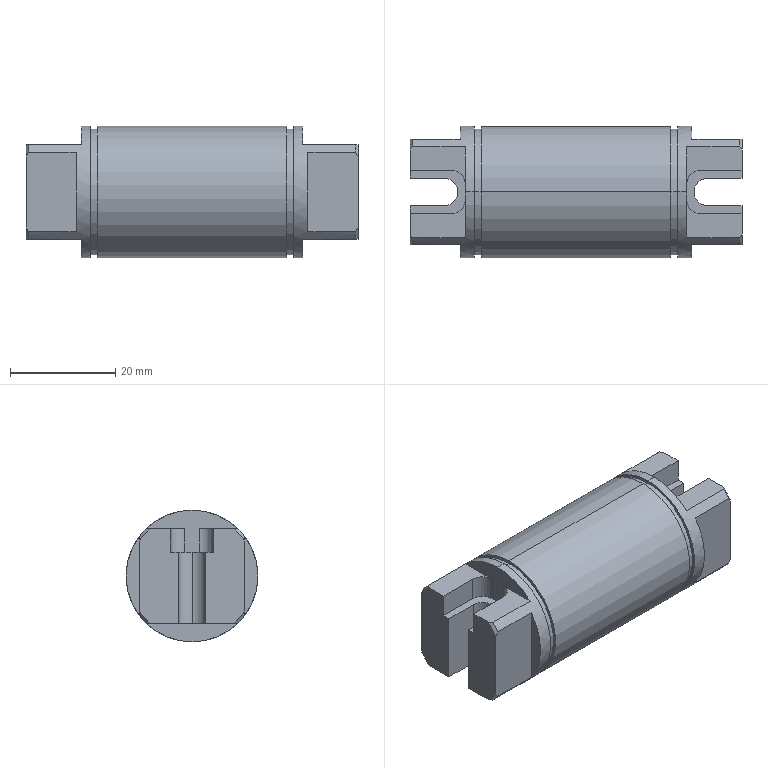Part | SolidWorks | features BaseBody 1 | 1 solid | 61 faces | box 63 x 25 x 25 mm | volume 26140 mm3 | plane 36 | cylinder 17 | cone 8 | commonest cylinder face diameters 5.2 x7 25 x6 23.9 x4